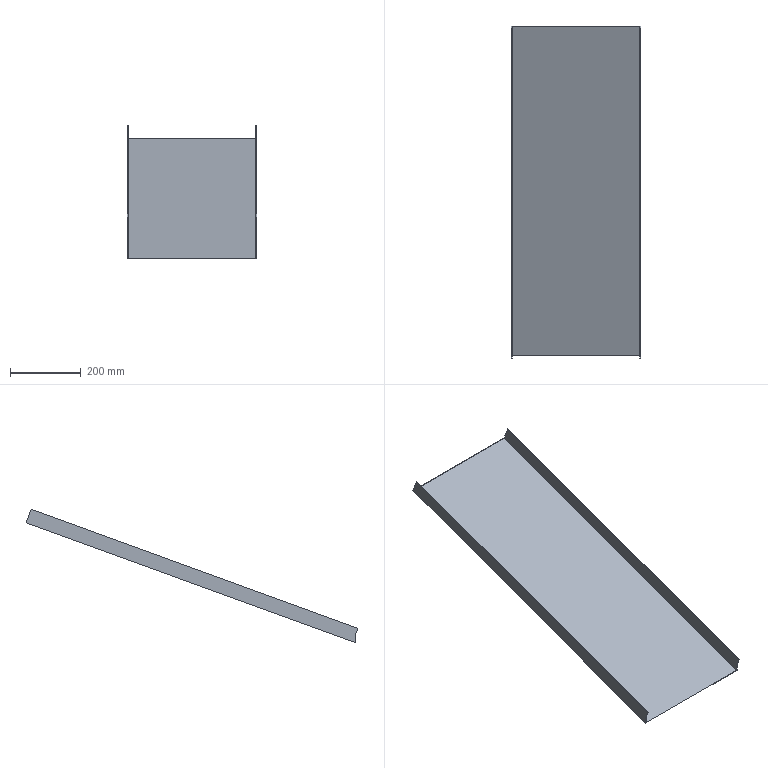Part | NX | features solid 2 | 1 solid | 12 faces | box 365 x 936.307 x 376.531 mm | volume 517909 mm3 | plane 12
STEP:
#1=CARTESIAN_POINT('',(-370.486,-1050.,-590.939));
#2=VERTEX_POINT('',#1);
#3=CARTESIAN_POINT('',(-731.486,-1050.,-590.939));
#4=VERTEX_POINT('',#3);
#5=CARTESIAN_POINT('',(-368.486,-1050.,-590.939));
#6=DIRECTION('',(1.,0.,0.));
#7=VECTOR('',#6,1000.);
#8=LINE('',#5,#7);
#9=EDGE_CURVE('',#2,#4,#8,.F.);
#10=ORIENTED_EDGE('',*,*,#9,.F.);
#11=CARTESIAN_POINT('',(-370.486,-121.685,-253.06));
#12=VERTEX_POINT('',#11);
#13=CARTESIAN_POINT('',(-370.486,-121.685,-253.06));
#14=DIRECTION('',(0.,-0.9397,-0.342));
#15=VECTOR('',#14,1000.);
#16=LINE('',#13,#15);
#17=EDGE_CURVE('',#12,#2,#16,.T.);
#18=ORIENTED_EDGE('',*,*,#17,.F.);
#19=CARTESIAN_POINT('',(-731.486,-121.685,-253.06));
#20=VERTEX_POINT('',#19);
#21=CARTESIAN_POINT('',(-368.486,-121.685,-253.06));
#22=DIRECTION('',(-1.,0.,0.));
#23=VECTOR('',#22,1000.);
#24=LINE('',#21,#23);
#25=EDGE_CURVE('',#20,#12,#24,.F.);
#26=ORIENTED_EDGE('',*,*,#25,.F.);
#27=CARTESIAN_POINT('',(-731.486,-121.685,-253.06));
#28=DIRECTION('',(0.,-0.9397,-0.342));
#29=VECTOR('',#28,1000.);
#30=LINE('',#27,#29);
#31=EDGE_CURVE('',#20,#4,#30,.T.);
#32=ORIENTED_EDGE('',*,*,#31,.T.);
#33=EDGE_LOOP('',(#10,#18,#26,#32));
#34=FACE_BOUND('',#33,.T.);
#35=CARTESIAN_POINT('',(-368.486,-496.391,-389.442));
#36=DIRECTION('',(0.,-0.342,0.9397));
#37=DIRECTION('',(0.,0.9397,0.342));
#38=AXIS2_PLACEMENT_3D('',#35,#36,#37);
#39=PLANE('',#38);
#40=ADVANCED_FACE('',(#34),#39,.T.);
#41=CARTESIAN_POINT('',(-733.486,-121.343,-254.));
#42=VERTEX_POINT('',#41);
#43=CARTESIAN_POINT('',(-733.486,-135.366,-215.473));
#44=VERTEX_POINT('',#43);
#45=CARTESIAN_POINT('',(-733.486,-121.343,-254.));
#46=DIRECTION('',(0.,-0.342,0.9397));
#47=VECTOR('',#46,1000.);
#48=LINE('',#45,#47);
#49=EDGE_CURVE('',#42,#44,#48,.T.);
#50=ORIENTED_EDGE('',*,*,#49,.T.);
#51=CARTESIAN_POINT('',(-731.486,-135.366,-215.473));
#52=VERTEX_POINT('',#51);
#53=CARTESIAN_POINT('',(-733.486,-135.366,-215.473));
#54=DIRECTION('',(1.,0.,0.));
#55=VECTOR('',#54,1000.);
#56=LINE('',#53,#55);
#57=EDGE_CURVE('',#44,#52,#56,.T.);
#58=ORIENTED_EDGE('',*,*,#57,.T.);
#59=CARTESIAN_POINT('',(-731.486,-135.366,-215.473));
#60=DIRECTION('',(0.,0.342,-0.9397));
#61=VECTOR('',#60,1000.);
#62=LINE('',#59,#61);
#63=EDGE_CURVE('',#52,#20,#62,.T.);
#64=ORIENTED_EDGE('',*,*,#63,.T.);
#65=ORIENTED_EDGE('',*,*,#25,.T.);
#66=CARTESIAN_POINT('',(-370.486,-135.366,-215.473));
#67=VERTEX_POINT('',#66);
#68=CARTESIAN_POINT('',(-370.486,-135.366,-215.473));
#69=DIRECTION('',(0.,0.342,-0.9397));
#70=VECTOR('',#69,1000.);
#71=LINE('',#68,#70);
#72=EDGE_CURVE('',#67,#12,#71,.T.);
#73=ORIENTED_EDGE('',*,*,#72,.F.);
#74=CARTESIAN_POINT('',(-368.486,-135.366,-215.473));
#75=VERTEX_POINT('',#74);
#76=CARTESIAN_POINT('',(-368.486,-135.366,-215.473));
#77=DIRECTION('',(1.,0.,0.));
#78=VECTOR('',#77,1000.);
#79=LINE('',#76,#78);
#80=EDGE_CURVE('',#75,#67,#79,.F.);
#81=ORIENTED_EDGE('',*,*,#80,.F.);
#82=CARTESIAN_POINT('',(-368.486,-121.343,-254.));
#83=VERTEX_POINT('',#82);
#84=CARTESIAN_POINT('',(-368.486,-121.343,-254.));
#85=DIRECTION('',(0.,-0.342,0.9397));
#86=VECTOR('',#85,1000.);
#87=LINE('',#84,#86);
#88=EDGE_CURVE('',#83,#75,#87,.T.);
#89=ORIENTED_EDGE('',*,*,#88,.F.);
#90=CARTESIAN_POINT('',(-368.486,-121.343,-254.));
#91=DIRECTION('',(-1.,0.,0.));
#92=VECTOR('',#91,1000.);
#93=LINE('',#90,#92);
#94=EDGE_CURVE('',#42,#83,#93,.F.);
#95=ORIENTED_EDGE('',*,*,#94,.F.);
#96=EDGE_LOOP('',(#50,#58,#64,#65,#73,#81,#89,#95));
#97=FACE_BOUND('',#96,.T.);
#98=CARTESIAN_POINT('',(-368.486,-121.343,-254.));
#99=DIRECTION('',(0.,-0.9397,-0.342));
#100=DIRECTION('',(0.,0.342,-0.9397));
#101=AXIS2_PLACEMENT_3D('',#98,#99,#100);
#102=PLANE('',#101);
#103=ADVANCED_FACE('',(#97),#102,.F.);
#104=CARTESIAN_POINT('',(-733.486,-1050.,-592.003));
#105=VERTEX_POINT('',#104);
#106=CARTESIAN_POINT('',(-733.486,-1050.,-572.175));
#107=VERTEX_POINT('',#106);
#108=CARTESIAN_POINT('',(-733.486,-1050.,-519.));
#109=DIRECTION('',(0.,0.,-1.));
#110=VECTOR('',#109,1000.);
#111=LINE('',#108,#110);
#112=EDGE_CURVE('',#105,#107,#111,.F.);
#113=ORIENTED_EDGE('',*,*,#112,.T.);
#114=CARTESIAN_POINT('',(-733.486,-1057.65,-551.157));
#115=VERTEX_POINT('',#114);
#116=CARTESIAN_POINT('',(-733.486,-1057.65,-551.157));
#117=DIRECTION('',(0.,0.342,-0.9397));
#118=VECTOR('',#117,1000.);
#119=LINE('',#116,#118);
#120=EDGE_CURVE('',#115,#107,#119,.T.);
#121=ORIENTED_EDGE('',*,*,#120,.F.);
#122=CARTESIAN_POINT('',(-733.486,-135.366,-215.473));
#123=DIRECTION('',(0.,-0.9397,-0.342));
#124=VECTOR('',#123,1000.);
#125=LINE('',#122,#124);
#126=EDGE_CURVE('',#44,#115,#125,.T.);
#127=ORIENTED_EDGE('',*,*,#126,.F.);
#128=ORIENTED_EDGE('',*,*,#49,.F.);
#129=CARTESIAN_POINT('',(-733.486,-496.049,-390.382));
#130=DIRECTION('',(0.,-0.9397,-0.342));
#131=VECTOR('',#130,1000.);
#132=LINE('',#129,#131);
#133=EDGE_CURVE('',#42,#105,#132,.T.);
#134=ORIENTED_EDGE('',*,*,#133,.T.);
#135=EDGE_LOOP('',(#113,#121,#127,#128,#134));
#136=FACE_BOUND('',#135,.T.);
#137=CARTESIAN_POINT('',(-733.486,-496.049,-390.382));
#138=DIRECTION('',(-1.,0.,0.));
#139=DIRECTION('',(0.,-1.,0.));
#140=AXIS2_PLACEMENT_3D('',#137,#138,#139);
#141=PLANE('',#140);
#142=ADVANCED_FACE('',(#136),#141,.T.);
#143=CARTESIAN_POINT('',(-368.486,-1050.,-572.175));
#144=VERTEX_POINT('',#143);
#145=CARTESIAN_POINT('',(-370.486,-1050.,-572.175));
#146=VERTEX_POINT('',#145);
#147=CARTESIAN_POINT('',(-368.486,-1050.,-572.175));
#148=DIRECTION('',(-1.,0.,0.));
#149=VECTOR('',#148,1000.);
#150=LINE('',#147,#149);
#151=EDGE_CURVE('',#144,#146,#150,.T.);
#152=ORIENTED_EDGE('',*,*,#151,.T.);
#153=CARTESIAN_POINT('',(-370.486,-1050.,-519.));
#154=DIRECTION('',(0.,0.,1.));
#155=VECTOR('',#154,1000.);
#156=LINE('',#153,#155);
#157=EDGE_CURVE('',#146,#2,#156,.F.);
#158=ORIENTED_EDGE('',*,*,#157,.T.);
#159=ORIENTED_EDGE('',*,*,#9,.T.);
#160=CARTESIAN_POINT('',(-731.486,-1050.,-572.175));
#161=VERTEX_POINT('',#160);
#162=CARTESIAN_POINT('',(-731.486,-1050.,-519.));
#163=DIRECTION('',(0.,0.,1.));
#164=VECTOR('',#163,1000.);
#165=LINE('',#162,#164);
#166=EDGE_CURVE('',#161,#4,#165,.F.);
#167=ORIENTED_EDGE('',*,*,#166,.F.);
#168=CARTESIAN_POINT('',(-733.486,-1050.,-572.175));
#169=DIRECTION('',(-1.,0.,0.));
#170=VECTOR('',#169,1000.);
#171=LINE('',#168,#170);
#172=EDGE_CURVE('',#107,#161,#171,.F.);
#173=ORIENTED_EDGE('',*,*,#172,.F.);
#174=ORIENTED_EDGE('',*,*,#112,.F.);
#175=CARTESIAN_POINT('',(-368.486,-1050.,-592.003));
#176=VERTEX_POINT('',#175);
#177=CARTESIAN_POINT('',(-368.486,-1050.,-592.003));
#178=DIRECTION('',(1.,0.,0.));
#179=VECTOR('',#178,1000.);
#180=LINE('',#177,#179);
#181=EDGE_CURVE('',#176,#105,#180,.F.);
#182=ORIENTED_EDGE('',*,*,#181,.F.);
#183=CARTESIAN_POINT('',(-368.486,-1050.,-519.));
#184=DIRECTION('',(0.,0.,-1.));
#185=VECTOR('',#184,1000.);
#186=LINE('',#183,#185);
#187=EDGE_CURVE('',#176,#144,#186,.F.);
#188=ORIENTED_EDGE('',*,*,#187,.T.);
#189=EDGE_LOOP('',(#152,#158,#159,#167,#173,#174,#182,#188));
#190=FACE_BOUND('',#189,.T.);
#191=CARTESIAN_POINT('',(750.,-1050.,-519.));
#192=DIRECTION('',(0.,-1.,0.));
#193=DIRECTION('',(1.,0.,0.));
#194=AXIS2_PLACEMENT_3D('',#191,#192,#193);
#195=PLANE('',#194);
#196=ADVANCED_FACE('',(#190),#195,.T.);
#197=ORIENTED_EDGE('',*,*,#88,.T.);
#198=CARTESIAN_POINT('',(-368.486,-1057.65,-551.157));
#199=VERTEX_POINT('',#198);
#200=CARTESIAN_POINT('',(-368.486,-135.366,-215.473));
#201=DIRECTION('',(0.,-0.9397,-0.342));
#202=VECTOR('',#201,1000.);
#203=LINE('',#200,#202);
#204=EDGE_CURVE('',#75,#199,#203,.T.);
#205=ORIENTED_EDGE('',*,*,#204,.T.);
#206=CARTESIAN_POINT('',(-368.486,-1043.627,-589.684));
#207=DIRECTION('',(0.,-0.342,0.9397));
#208=VECTOR('',#207,1000.);
#209=LINE('',#206,#208);
#210=EDGE_CURVE('',#199,#144,#209,.F.);
#211=ORIENTED_EDGE('',*,*,#210,.T.);
#212=ORIENTED_EDGE('',*,*,#187,.F.);
#213=CARTESIAN_POINT('',(-368.486,-496.049,-390.382));
#214=DIRECTION('',(0.,-0.9397,-0.342));
#215=VECTOR('',#214,1000.);
#216=LINE('',#213,#215);
#217=EDGE_CURVE('',#83,#176,#216,.T.);
#218=ORIENTED_EDGE('',*,*,#217,.F.);
#219=EDGE_LOOP('',(#197,#205,#211,#212,#218));
#220=FACE_BOUND('',#219,.T.);
#221=CARTESIAN_POINT('',(-368.486,-496.049,-390.382));
#222=DIRECTION('',(-1.,0.,0.));
#223=DIRECTION('',(0.,0.,1.));
#224=AXIS2_PLACEMENT_3D('',#221,#222,#223);
#225=PLANE('',#224);
#226=ADVANCED_FACE('',(#220),#225,.F.);
#227=ORIENTED_EDGE('',*,*,#94,.T.);
#228=ORIENTED_EDGE('',*,*,#217,.T.);
#229=ORIENTED_EDGE('',*,*,#181,.T.);
#230=ORIENTED_EDGE('',*,*,#133,.F.);
#231=EDGE_LOOP('',(#227,#228,#229,#230));
#232=FACE_BOUND('',#231,.T.);
#233=CARTESIAN_POINT('',(-368.486,-496.049,-390.382));
#234=DIRECTION('',(0.,-0.342,0.9397));
#235=DIRECTION('',(0.,0.9397,0.342));
#236=AXIS2_PLACEMENT_3D('',#233,#234,#235);
#237=PLANE('',#236);
#238=ADVANCED_FACE('',(#232),#237,.F.);
#239=ORIENTED_EDGE('',*,*,#57,.F.);
#240=ORIENTED_EDGE('',*,*,#126,.T.);
#241=CARTESIAN_POINT('',(-731.486,-1057.65,-551.157));
#242=VERTEX_POINT('',#241);
#243=CARTESIAN_POINT('',(-733.486,-1057.65,-551.157));
#244=DIRECTION('',(1.,0.,0.));
#245=VECTOR('',#244,1000.);
#246=LINE('',#243,#245);
#247=EDGE_CURVE('',#115,#242,#246,.T.);
#248=ORIENTED_EDGE('',*,*,#247,.T.);
#249=CARTESIAN_POINT('',(-731.486,-135.366,-215.473));
#250=DIRECTION('',(0.,-0.9397,-0.342));
#251=VECTOR('',#250,1000.);
#252=LINE('',#249,#251);
#253=EDGE_CURVE('',#52,#242,#252,.T.);
#254=ORIENTED_EDGE('',*,*,#253,.F.);
#255=EDGE_LOOP('',(#239,#240,#248,#254));
#256=FACE_BOUND('',#255,.T.);
#257=CARTESIAN_POINT('',(-733.486,-135.366,-215.473));
#258=DIRECTION('',(0.,-0.342,0.9397));
#259=DIRECTION('',(0.,-0.9397,-0.342));
#260=AXIS2_PLACEMENT_3D('',#257,#258,#259);
#261=PLANE('',#260);
#262=ADVANCED_FACE('',(#256),#261,.T.);
#263=ORIENTED_EDGE('',*,*,#247,.F.);
#264=ORIENTED_EDGE('',*,*,#120,.T.);
#265=ORIENTED_EDGE('',*,*,#172,.T.);
#266=CARTESIAN_POINT('',(-731.486,-1057.65,-551.157));
#267=DIRECTION('',(0.,0.342,-0.9397));
#268=VECTOR('',#267,1000.);
#269=LINE('',#266,#268);
#270=EDGE_CURVE('',#242,#161,#269,.T.);
#271=ORIENTED_EDGE('',*,*,#270,.F.);
#272=EDGE_LOOP('',(#263,#264,#265,#271));
#273=FACE_BOUND('',#272,.T.);
#274=CARTESIAN_POINT('',(-733.486,-1057.65,-551.157));
#275=DIRECTION('',(0.,-0.9397,-0.342));
#276=DIRECTION('',(0.,0.342,-0.9397));
#277=AXIS2_PLACEMENT_3D('',#274,#275,#276);
#278=PLANE('',#277);
#279=ADVANCED_FACE('',(#273),#278,.T.);
#280=ORIENTED_EDGE('',*,*,#31,.F.);
#281=ORIENTED_EDGE('',*,*,#63,.F.);
#282=ORIENTED_EDGE('',*,*,#253,.T.);
#283=ORIENTED_EDGE('',*,*,#270,.T.);
#284=ORIENTED_EDGE('',*,*,#166,.T.);
#285=EDGE_LOOP('',(#280,#281,#282,#283,#284));
#286=FACE_BOUND('',#285,.T.);
#287=CARTESIAN_POINT('',(-731.486,-135.366,-215.473));
#288=DIRECTION('',(1.,0.,0.));
#289=DIRECTION('',(0.,1.,0.));
#290=AXIS2_PLACEMENT_3D('',#287,#288,#289);
#291=PLANE('',#290);
#292=ADVANCED_FACE('',(#286),#291,.T.);
#293=ORIENTED_EDGE('',*,*,#80,.T.);
#294=CARTESIAN_POINT('',(-370.486,-1057.65,-551.157));
#295=VERTEX_POINT('',#294);
#296=CARTESIAN_POINT('',(-370.486,-135.366,-215.473));
#297=DIRECTION('',(0.,-0.9397,-0.342));
#298=VECTOR('',#297,1000.);
#299=LINE('',#296,#298);
#300=EDGE_CURVE('',#67,#295,#299,.T.);
#301=ORIENTED_EDGE('',*,*,#300,.T.);
#302=CARTESIAN_POINT('',(-368.486,-1057.65,-551.157));
#303=DIRECTION('',(-1.,0.,0.));
#304=VECTOR('',#303,1000.);
#305=LINE('',#302,#304);
#306=EDGE_CURVE('',#199,#295,#305,.T.);
#307=ORIENTED_EDGE('',*,*,#306,.F.);
#308=ORIENTED_EDGE('',*,*,#204,.F.);
#309=EDGE_LOOP('',(#293,#301,#307,#308));
#310=FACE_BOUND('',#309,.T.);
#311=CARTESIAN_POINT('',(-368.486,-135.366,-215.473));
#312=DIRECTION('',(0.,-0.342,0.9397));
#313=DIRECTION('',(0.,-0.9397,-0.342));
#314=AXIS2_PLACEMENT_3D('',#311,#312,#313);
#315=PLANE('',#314);
#316=ADVANCED_FACE('',(#310),#315,.T.);
#317=ORIENTED_EDGE('',*,*,#306,.T.);
#318=CARTESIAN_POINT('',(-370.486,-1057.65,-551.157));
#319=DIRECTION('',(0.,-0.342,0.9397));
#320=VECTOR('',#319,1000.);
#321=LINE('',#318,#320);
#322=EDGE_CURVE('',#295,#146,#321,.F.);
#323=ORIENTED_EDGE('',*,*,#322,.T.);
#324=ORIENTED_EDGE('',*,*,#151,.F.);
#325=ORIENTED_EDGE('',*,*,#210,.F.);
#326=EDGE_LOOP('',(#317,#323,#324,#325));
#327=FACE_BOUND('',#326,.T.);
#328=CARTESIAN_POINT('',(-368.486,-1057.65,-551.157));
#329=DIRECTION('',(0.,-0.9397,-0.342));
#330=DIRECTION('',(0.,0.342,-0.9397));
#331=AXIS2_PLACEMENT_3D('',#328,#329,#330);
#332=PLANE('',#331);
#333=ADVANCED_FACE('',(#327),#332,.T.);
#334=ORIENTED_EDGE('',*,*,#17,.T.);
#335=ORIENTED_EDGE('',*,*,#157,.F.);
#336=ORIENTED_EDGE('',*,*,#322,.F.);
#337=ORIENTED_EDGE('',*,*,#300,.F.);
#338=ORIENTED_EDGE('',*,*,#72,.T.);
#339=EDGE_LOOP('',(#334,#335,#336,#337,#338));
#340=FACE_BOUND('',#339,.T.);
#341=CARTESIAN_POINT('',(-370.486,-135.366,-215.473));
#342=DIRECTION('',(1.,0.,0.));
#343=DIRECTION('',(0.,0.,-1.));
#344=AXIS2_PLACEMENT_3D('',#341,#342,#343);
#345=PLANE('',#344);
#346=ADVANCED_FACE('',(#340),#345,.F.);
#347=CLOSED_SHELL('',(#40,#103,#142,#196,#226,#238,#262,#279,#292,#316,#333,#346));
#348=MANIFOLD_SOLID_BREP('',#347);
#349=(LENGTH_UNIT()NAMED_UNIT(*)SI_UNIT(.MILLI.,.METRE.));
#350=UNCERTAINTY_MEASURE_WITH_UNIT(LENGTH_MEASURE(0.00001),#349,'','');
#351=(NAMED_UNIT(*)PLANE_ANGLE_UNIT()SI_UNIT($,.RADIAN.));
#352=(NAMED_UNIT(*)SI_UNIT($,.STERADIAN.)SOLID_ANGLE_UNIT());
#353=(GEOMETRIC_REPRESENTATION_CONTEXT(3)GLOBAL_UNCERTAINTY_ASSIGNED_CONTEXT((#350))GLOBAL_UNIT_ASSIGNED_CONTEXT((#349,#351,#352))REPRESENTATION_CONTEXT('',''));
#354=ADVANCED_BREP_SHAPE_REPRESENTATION('',(#348),#353);